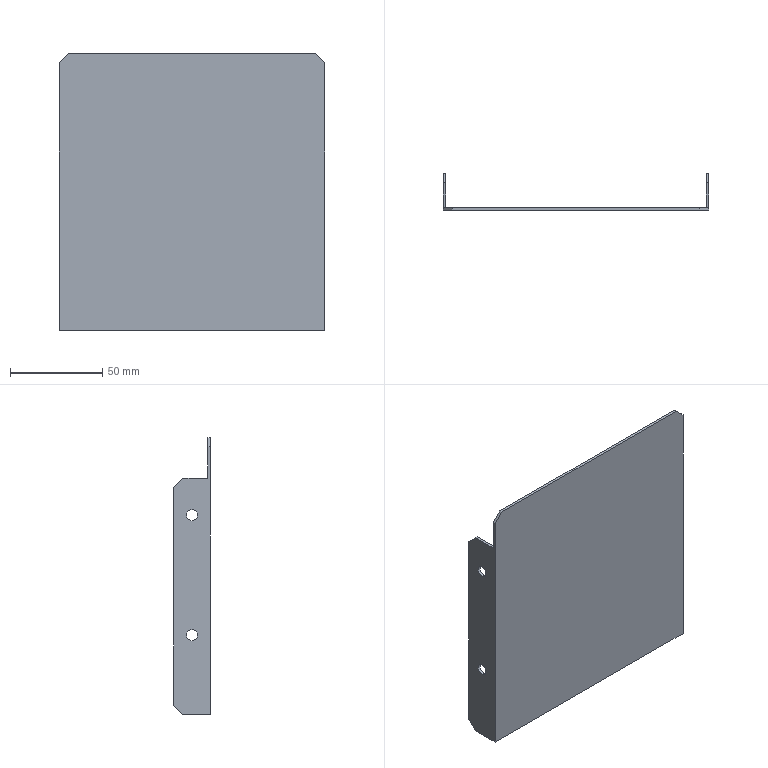Part | STEP file | MANG DAN PHOI CO LOGO | 1 solid | 26 faces | box 144 x 20 x 150 mm | volume 39222 mm3 | plane 18 | cylinder 8 | commonest cylinder face diameters 6 x8